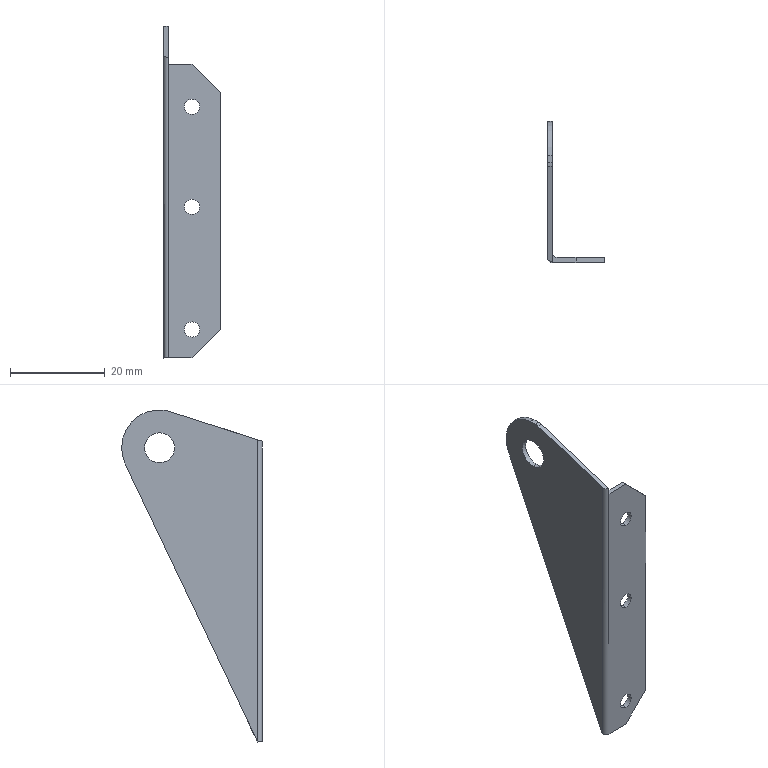Part | SolidWorks | features BaseBody 1 | 1 solid | 24 faces | box 12 x 29.68 x 70 mm | volume 1722 mm3 | cylinder 12 | plane 12 | commonest cylinder face diameters 3.2 x6 2 x2 6.35 x2 16 x2
STEP:
#1=CARTESIAN_POINT('',(6.,0.,33.461));
#2=VERTEX_POINT('',#1);
#3=CARTESIAN_POINT('',(6.,0.,30.261));
#4=VERTEX_POINT('',#3);
#5=CARTESIAN_POINT('',(6.,0.,31.861));
#6=DIRECTION('',(0.,-1.,0.));
#7=DIRECTION('',(0.,0.,1.));
#8=AXIS2_PLACEMENT_3D('',#5,#6,#7);
#9=CIRCLE('',#8,1.6);
#10=EDGE_CURVE('',#2,#4,#9,.T.);
#11=ORIENTED_EDGE('',*,*,#10,.T.);
#12=CARTESIAN_POINT('',(6.,1.,30.261));
#13=VERTEX_POINT('',#12);
#14=CARTESIAN_POINT('',(6.,0.,30.261));
#15=DIRECTION('',(0.,1.,0.));
#16=VECTOR('',#15,1000.);
#17=LINE('',#14,#16);
#18=EDGE_CURVE('',#4,#13,#17,.T.);
#19=ORIENTED_EDGE('',*,*,#18,.T.);
#20=CARTESIAN_POINT('',(6.,1.,33.461));
#21=VERTEX_POINT('',#20);
#22=CARTESIAN_POINT('',(6.,1.,31.861));
#23=DIRECTION('',(0.,1.,0.));
#24=DIRECTION('',(0.,0.,1.));
#25=AXIS2_PLACEMENT_3D('',#22,#23,#24);
#26=CIRCLE('',#25,1.6);
#27=EDGE_CURVE('',#13,#21,#26,.T.);
#28=ORIENTED_EDGE('',*,*,#27,.T.);
#29=CARTESIAN_POINT('',(6.,0.,33.461));
#30=DIRECTION('',(0.,1.,0.));
#31=VECTOR('',#30,1000.);
#32=LINE('',#29,#31);
#33=EDGE_CURVE('',#2,#21,#32,.T.);
#34=ORIENTED_EDGE('',*,*,#33,.F.);
#35=EDGE_LOOP('',(#11,#19,#28,#34));
#36=FACE_OUTER_BOUND('',#35,.T.);
#37=CARTESIAN_POINT('',(6.,0.,31.861));
#38=DIRECTION('',(0.,1.,0.));
#39=DIRECTION('',(0.,0.,1.));
#40=AXIS2_PLACEMENT_3D('',#37,#38,#39);
#41=CYLINDRICAL_SURFACE('',#40,1.6);
#42=ADVANCED_FACE('',(#36),#41,.F.);
#43=CARTESIAN_POINT('',(6.,0.,54.587));
#44=VERTEX_POINT('',#43);
#45=CARTESIAN_POINT('',(6.,0.,51.387));
#46=VERTEX_POINT('',#45);
#47=CARTESIAN_POINT('',(6.,0.,52.987));
#48=DIRECTION('',(0.,-1.,0.));
#49=DIRECTION('',(0.,0.,1.));
#50=AXIS2_PLACEMENT_3D('',#47,#48,#49);
#51=CIRCLE('',#50,1.6);
#52=EDGE_CURVE('',#44,#46,#51,.T.);
#53=ORIENTED_EDGE('',*,*,#52,.T.);
#54=CARTESIAN_POINT('',(6.,1.,51.387));
#55=VERTEX_POINT('',#54);
#56=CARTESIAN_POINT('',(6.,0.,51.387));
#57=DIRECTION('',(0.,1.,0.));
#58=VECTOR('',#57,1000.);
#59=LINE('',#56,#58);
#60=EDGE_CURVE('',#46,#55,#59,.T.);
#61=ORIENTED_EDGE('',*,*,#60,.T.);
#62=CARTESIAN_POINT('',(6.,1.,54.587));
#63=VERTEX_POINT('',#62);
#64=CARTESIAN_POINT('',(6.,1.,52.987));
#65=DIRECTION('',(0.,1.,0.));
#66=DIRECTION('',(0.,0.,1.));
#67=AXIS2_PLACEMENT_3D('',#64,#65,#66);
#68=CIRCLE('',#67,1.6);
#69=EDGE_CURVE('',#55,#63,#68,.T.);
#70=ORIENTED_EDGE('',*,*,#69,.T.);
#71=CARTESIAN_POINT('',(6.,0.,54.587));
#72=DIRECTION('',(0.,1.,0.));
#73=VECTOR('',#72,1000.);
#74=LINE('',#71,#73);
#75=EDGE_CURVE('',#44,#63,#74,.T.);
#76=ORIENTED_EDGE('',*,*,#75,.F.);
#77=EDGE_LOOP('',(#53,#61,#70,#76));
#78=FACE_OUTER_BOUND('',#77,.T.);
#79=CARTESIAN_POINT('',(6.,0.,52.987));
#80=DIRECTION('',(0.,1.,0.));
#81=DIRECTION('',(0.,0.,1.));
#82=AXIS2_PLACEMENT_3D('',#79,#80,#81);
#83=CYLINDRICAL_SURFACE('',#82,1.6);
#84=ADVANCED_FACE('',(#78),#83,.F.);
#85=CARTESIAN_POINT('',(6.,0.,7.6));
#86=VERTEX_POINT('',#85);
#87=CARTESIAN_POINT('',(6.,0.,4.4));
#88=VERTEX_POINT('',#87);
#89=CARTESIAN_POINT('',(6.,0.,6.));
#90=DIRECTION('',(0.,-1.,0.));
#91=DIRECTION('',(0.,0.,1.));
#92=AXIS2_PLACEMENT_3D('',#89,#90,#91);
#93=CIRCLE('',#92,1.6);
#94=EDGE_CURVE('',#86,#88,#93,.T.);
#95=ORIENTED_EDGE('',*,*,#94,.T.);
#96=CARTESIAN_POINT('',(6.,1.,4.4));
#97=VERTEX_POINT('',#96);
#98=CARTESIAN_POINT('',(6.,0.,4.4));
#99=DIRECTION('',(0.,1.,0.));
#100=VECTOR('',#99,1000.);
#101=LINE('',#98,#100);
#102=EDGE_CURVE('',#88,#97,#101,.T.);
#103=ORIENTED_EDGE('',*,*,#102,.T.);
#104=CARTESIAN_POINT('',(6.,1.,7.6));
#105=VERTEX_POINT('',#104);
#106=CARTESIAN_POINT('',(6.,1.,6.));
#107=DIRECTION('',(0.,1.,0.));
#108=DIRECTION('',(0.,0.,1.));
#109=AXIS2_PLACEMENT_3D('',#106,#107,#108);
#110=CIRCLE('',#109,1.6);
#111=EDGE_CURVE('',#97,#105,#110,.T.);
#112=ORIENTED_EDGE('',*,*,#111,.T.);
#113=CARTESIAN_POINT('',(6.,0.,7.6));
#114=DIRECTION('',(0.,1.,0.));
#115=VECTOR('',#114,1000.);
#116=LINE('',#113,#115);
#117=EDGE_CURVE('',#86,#105,#116,.T.);
#118=ORIENTED_EDGE('',*,*,#117,.F.);
#119=EDGE_LOOP('',(#95,#103,#112,#118));
#120=FACE_OUTER_BOUND('',#119,.T.);
#121=CARTESIAN_POINT('',(6.,0.,6.));
#122=DIRECTION('',(0.,1.,0.));
#123=DIRECTION('',(0.,0.,1.));
#124=AXIS2_PLACEMENT_3D('',#121,#122,#123);
#125=CYLINDRICAL_SURFACE('',#124,1.6);
#126=ADVANCED_FACE('',(#120),#125,.F.);
#127=CARTESIAN_POINT('',(0.,21.68,58.856));
#128=VERTEX_POINT('',#127);
#129=CARTESIAN_POINT('',(0.,21.68,65.206));
#130=VERTEX_POINT('',#129);
#131=CARTESIAN_POINT('',(0.,21.68,62.031));
#132=DIRECTION('',(-1.,0.,0.));
#133=DIRECTION('',(0.,0.,-1.));
#134=AXIS2_PLACEMENT_3D('',#131,#132,#133);
#135=CIRCLE('',#134,3.175);
#136=EDGE_CURVE('',#128,#130,#135,.T.);
#137=ORIENTED_EDGE('',*,*,#136,.T.);
#138=CARTESIAN_POINT('',(1.,21.68,65.206));
#139=VERTEX_POINT('',#138);
#140=CARTESIAN_POINT('',(0.,21.68,65.206));
#141=DIRECTION('',(1.,0.,0.));
#142=VECTOR('',#141,1000.);
#143=LINE('',#140,#142);
#144=EDGE_CURVE('',#130,#139,#143,.T.);
#145=ORIENTED_EDGE('',*,*,#144,.T.);
#146=CARTESIAN_POINT('',(1.,21.68,58.856));
#147=VERTEX_POINT('',#146);
#148=CARTESIAN_POINT('',(1.,21.68,62.031));
#149=DIRECTION('',(1.,0.,0.));
#150=DIRECTION('',(0.,0.,-1.));
#151=AXIS2_PLACEMENT_3D('',#148,#149,#150);
#152=CIRCLE('',#151,3.175);
#153=EDGE_CURVE('',#139,#147,#152,.T.);
#154=ORIENTED_EDGE('',*,*,#153,.T.);
#155=CARTESIAN_POINT('',(0.,21.68,58.856));
#156=DIRECTION('',(1.,0.,0.));
#157=VECTOR('',#156,1000.);
#158=LINE('',#155,#157);
#159=EDGE_CURVE('',#128,#147,#158,.T.);
#160=ORIENTED_EDGE('',*,*,#159,.F.);
#161=EDGE_LOOP('',(#137,#145,#154,#160));
#162=FACE_OUTER_BOUND('',#161,.T.);
#163=CARTESIAN_POINT('',(0.,21.68,62.031));
#164=DIRECTION('',(1.,0.,0.));
#165=DIRECTION('',(0.,0.,-1.));
#166=AXIS2_PLACEMENT_3D('',#163,#164,#165);
#167=CYLINDRICAL_SURFACE('',#166,3.175);
#168=ADVANCED_FACE('',(#162),#167,.F.);
#169=ORIENTED_EDGE('',*,*,#18,.F.);
#170=CARTESIAN_POINT('',(6.,0.,31.861));
#171=DIRECTION('',(0.,-1.,0.));
#172=DIRECTION('',(0.,0.,1.));
#173=AXIS2_PLACEMENT_3D('',#170,#171,#172);
#174=CIRCLE('',#173,1.6);
#175=EDGE_CURVE('',#4,#2,#174,.T.);
#176=ORIENTED_EDGE('',*,*,#175,.T.);
#177=ORIENTED_EDGE('',*,*,#33,.T.);
#178=CARTESIAN_POINT('',(6.,1.,31.861));
#179=DIRECTION('',(0.,1.,0.));
#180=DIRECTION('',(0.,0.,1.));
#181=AXIS2_PLACEMENT_3D('',#178,#179,#180);
#182=CIRCLE('',#181,1.6);
#183=EDGE_CURVE('',#21,#13,#182,.T.);
#184=ORIENTED_EDGE('',*,*,#183,.T.);
#185=EDGE_LOOP('',(#169,#176,#177,#184));
#186=FACE_OUTER_BOUND('',#185,.T.);
#187=CARTESIAN_POINT('',(6.,0.,31.861));
#188=DIRECTION('',(0.,1.,0.));
#189=DIRECTION('',(0.,0.,1.));
#190=AXIS2_PLACEMENT_3D('',#187,#188,#189);
#191=CYLINDRICAL_SURFACE('',#190,1.6);
#192=ADVANCED_FACE('',(#186),#191,.F.);
#193=CARTESIAN_POINT('',(6.,1.,52.987));
#194=DIRECTION('',(0.,1.,0.));
#195=DIRECTION('',(0.,0.,1.));
#196=AXIS2_PLACEMENT_3D('',#193,#194,#195);
#197=CIRCLE('',#196,1.6);
#198=EDGE_CURVE('',#63,#55,#197,.T.);
#199=ORIENTED_EDGE('',*,*,#198,.F.);
#200=ORIENTED_EDGE('',*,*,#69,.F.);
#201=EDGE_LOOP('',(#199,#200));
#202=FACE_BOUND('',#201,.T.);
#203=CARTESIAN_POINT('',(6.,1.,6.));
#204=DIRECTION('',(0.,1.,0.));
#205=DIRECTION('',(0.,0.,1.));
#206=AXIS2_PLACEMENT_3D('',#203,#204,#205);
#207=CIRCLE('',#206,1.6);
#208=EDGE_CURVE('',#105,#97,#207,.T.);
#209=ORIENTED_EDGE('',*,*,#208,.F.);
#210=ORIENTED_EDGE('',*,*,#111,.F.);
#211=EDGE_LOOP('',(#209,#210));
#212=FACE_BOUND('',#211,.T.);
#213=ORIENTED_EDGE('',*,*,#183,.F.);
#214=ORIENTED_EDGE('',*,*,#27,.F.);
#215=EDGE_LOOP('',(#213,#214));
#216=FACE_BOUND('',#215,.T.);
#217=CARTESIAN_POINT('',(2.,1.,61.987));
#218=VERTEX_POINT('',#217);
#219=CARTESIAN_POINT('',(2.,1.,0.));
#220=VERTEX_POINT('',#219);
#221=CARTESIAN_POINT('',(2.,1.,30.994));
#222=DIRECTION('',(0.,0.,-1.));
#223=VECTOR('',#222,1000.);
#224=LINE('',#221,#223);
#225=EDGE_CURVE('',#218,#220,#224,.T.);
#226=ORIENTED_EDGE('',*,*,#225,.F.);
#227=CARTESIAN_POINT('',(6.,1.,61.987));
#228=VERTEX_POINT('',#227);
#229=CARTESIAN_POINT('',(7.,1.,61.987));
#230=DIRECTION('',(-1.,0.,0.));
#231=VECTOR('',#230,1000.);
#232=LINE('',#229,#231);
#233=EDGE_CURVE('',#228,#218,#232,.T.);
#234=ORIENTED_EDGE('',*,*,#233,.F.);
#235=CARTESIAN_POINT('',(12.,1.,55.987));
#236=VERTEX_POINT('',#235);
#237=CARTESIAN_POINT('',(12.,1.,55.987));
#238=DIRECTION('',(-0.7071,0.,0.7071));
#239=VECTOR('',#238,1000.);
#240=LINE('',#237,#239);
#241=EDGE_CURVE('',#236,#228,#240,.T.);
#242=ORIENTED_EDGE('',*,*,#241,.F.);
#243=CARTESIAN_POINT('',(12.,1.,6.));
#244=VERTEX_POINT('',#243);
#245=CARTESIAN_POINT('',(12.,1.,30.994));
#246=DIRECTION('',(0.,0.,1.));
#247=VECTOR('',#246,1000.);
#248=LINE('',#245,#247);
#249=EDGE_CURVE('',#244,#236,#248,.T.);
#250=ORIENTED_EDGE('',*,*,#249,.F.);
#251=CARTESIAN_POINT('',(6.,1.,0.));
#252=VERTEX_POINT('',#251);
#253=CARTESIAN_POINT('',(6.,1.,0.));
#254=DIRECTION('',(0.7071,0.,0.7071));
#255=VECTOR('',#254,1000.);
#256=LINE('',#253,#255);
#257=EDGE_CURVE('',#252,#244,#256,.T.);
#258=ORIENTED_EDGE('',*,*,#257,.F.);
#259=CARTESIAN_POINT('',(7.,1.,0.));
#260=DIRECTION('',(1.,0.,0.));
#261=VECTOR('',#260,1000.);
#262=LINE('',#259,#261);
#263=EDGE_CURVE('',#220,#252,#262,.T.);
#264=ORIENTED_EDGE('',*,*,#263,.F.);
#265=EDGE_LOOP('',(#226,#234,#242,#250,#258,#264));
#266=FACE_OUTER_BOUND('',#265,.T.);
#267=CARTESIAN_POINT('',(2.,1.,61.987));
#268=DIRECTION('',(0.,-1.,0.));
#269=DIRECTION('',(0.,0.,-1.));
#270=AXIS2_PLACEMENT_3D('',#267,#268,#269);
#271=PLANE('',#270);
#272=ADVANCED_FACE('',(#202,#212,#216,#266),#271,.F.);
#273=ORIENTED_EDGE('',*,*,#52,.F.);
#274=CARTESIAN_POINT('',(6.,0.,52.987));
#275=DIRECTION('',(0.,-1.,0.));
#276=DIRECTION('',(0.,0.,1.));
#277=AXIS2_PLACEMENT_3D('',#274,#275,#276);
#278=CIRCLE('',#277,1.6);
#279=EDGE_CURVE('',#46,#44,#278,.T.);
#280=ORIENTED_EDGE('',*,*,#279,.F.);
#281=EDGE_LOOP('',(#273,#280));
#282=FACE_BOUND('',#281,.T.);
#283=ORIENTED_EDGE('',*,*,#94,.F.);
#284=CARTESIAN_POINT('',(6.,0.,6.));
#285=DIRECTION('',(0.,-1.,0.));
#286=DIRECTION('',(0.,0.,1.));
#287=AXIS2_PLACEMENT_3D('',#284,#285,#286);
#288=CIRCLE('',#287,1.6);
#289=EDGE_CURVE('',#88,#86,#288,.T.);
#290=ORIENTED_EDGE('',*,*,#289,.F.);
#291=EDGE_LOOP('',(#283,#290));
#292=FACE_BOUND('',#291,.T.);
#293=ORIENTED_EDGE('',*,*,#10,.F.);
#294=ORIENTED_EDGE('',*,*,#175,.F.);
#295=EDGE_LOOP('',(#293,#294));
#296=FACE_BOUND('',#295,.T.);
#297=CARTESIAN_POINT('',(1.,0.,0.));
#298=VERTEX_POINT('',#297);
#299=CARTESIAN_POINT('',(1.,0.,61.987));
#300=VERTEX_POINT('',#299);
#301=CARTESIAN_POINT('',(1.,0.,30.994));
#302=DIRECTION('',(0.,0.,1.));
#303=VECTOR('',#302,1000.);
#304=LINE('',#301,#303);
#305=EDGE_CURVE('',#298,#300,#304,.T.);
#306=ORIENTED_EDGE('',*,*,#305,.F.);
#307=CARTESIAN_POINT('',(6.,0.,0.));
#308=VERTEX_POINT('',#307);
#309=CARTESIAN_POINT('',(6.5,0.,0.));
#310=DIRECTION('',(-1.,0.,0.));
#311=VECTOR('',#310,1000.);
#312=LINE('',#309,#311);
#313=EDGE_CURVE('',#308,#298,#312,.T.);
#314=ORIENTED_EDGE('',*,*,#313,.F.);
#315=CARTESIAN_POINT('',(12.,0.,6.));
#316=VERTEX_POINT('',#315);
#317=CARTESIAN_POINT('',(6.,0.,0.));
#318=DIRECTION('',(-0.7071,0.,-0.7071));
#319=VECTOR('',#318,1000.);
#320=LINE('',#317,#319);
#321=EDGE_CURVE('',#316,#308,#320,.T.);
#322=ORIENTED_EDGE('',*,*,#321,.F.);
#323=CARTESIAN_POINT('',(12.,0.,55.987));
#324=VERTEX_POINT('',#323);
#325=CARTESIAN_POINT('',(12.,0.,30.994));
#326=DIRECTION('',(0.,0.,-1.));
#327=VECTOR('',#326,1000.);
#328=LINE('',#325,#327);
#329=EDGE_CURVE('',#324,#316,#328,.T.);
#330=ORIENTED_EDGE('',*,*,#329,.F.);
#331=CARTESIAN_POINT('',(6.,0.,61.987));
#332=VERTEX_POINT('',#331);
#333=CARTESIAN_POINT('',(12.,0.,55.987));
#334=DIRECTION('',(0.7071,0.,-0.7071));
#335=VECTOR('',#334,1000.);
#336=LINE('',#333,#335);
#337=EDGE_CURVE('',#332,#324,#336,.T.);
#338=ORIENTED_EDGE('',*,*,#337,.F.);
#339=CARTESIAN_POINT('',(6.5,0.,61.987));
#340=DIRECTION('',(1.,0.,0.));
#341=VECTOR('',#340,1000.);
#342=LINE('',#339,#341);
#343=EDGE_CURVE('',#300,#332,#342,.T.);
#344=ORIENTED_EDGE('',*,*,#343,.F.);
#345=EDGE_LOOP('',(#306,#314,#322,#330,#338,#344));
#346=FACE_OUTER_BOUND('',#345,.T.);
#347=CARTESIAN_POINT('',(1.,0.,0.));
#348=DIRECTION('',(0.,1.,0.));
#349=DIRECTION('',(0.,0.,1.));
#350=AXIS2_PLACEMENT_3D('',#347,#348,#349);
#351=PLANE('',#350);
#352=ADVANCED_FACE('',(#282,#292,#296,#346),#351,.F.);
#353=ORIENTED_EDGE('',*,*,#60,.F.);
#354=ORIENTED_EDGE('',*,*,#279,.T.);
#355=ORIENTED_EDGE('',*,*,#75,.T.);
#356=ORIENTED_EDGE('',*,*,#198,.T.);
#357=EDGE_LOOP('',(#353,#354,#355,#356));
#358=FACE_OUTER_BOUND('',#357,.T.);
#359=CARTESIAN_POINT('',(6.,0.,52.987));
#360=DIRECTION('',(0.,1.,0.));
#361=DIRECTION('',(0.,0.,1.));
#362=AXIS2_PLACEMENT_3D('',#359,#360,#361);
#363=CYLINDRICAL_SURFACE('',#362,1.6);
#364=ADVANCED_FACE('',(#358),#363,.F.);
#365=ORIENTED_EDGE('',*,*,#102,.F.);
#366=ORIENTED_EDGE('',*,*,#289,.T.);
#367=ORIENTED_EDGE('',*,*,#117,.T.);
#368=ORIENTED_EDGE('',*,*,#208,.T.);
#369=EDGE_LOOP('',(#365,#366,#367,#368));
#370=FACE_OUTER_BOUND('',#369,.T.);
#371=CARTESIAN_POINT('',(6.,0.,6.));
#372=DIRECTION('',(0.,1.,0.));
#373=DIRECTION('',(0.,0.,1.));
#374=AXIS2_PLACEMENT_3D('',#371,#372,#373);
#375=CYLINDRICAL_SURFACE('',#374,1.6);
#376=ADVANCED_FACE('',(#370),#375,.F.);
#377=ORIENTED_EDGE('',*,*,#263,.T.);
#378=CARTESIAN_POINT('',(6.,0.5,0.));
#379=DIRECTION('',(0.,-1.,0.));
#380=VECTOR('',#379,1000.);
#381=LINE('',#378,#380);
#382=EDGE_CURVE('',#252,#308,#381,.T.);
#383=ORIENTED_EDGE('',*,*,#382,.T.);
#384=ORIENTED_EDGE('',*,*,#313,.T.);
#385=CARTESIAN_POINT('',(0.,1.,0.));
#386=VERTEX_POINT('',#385);
#387=CARTESIAN_POINT('',(1.,1.,0.));
#388=DIRECTION('',(0.,0.,-1.));
#389=DIRECTION('',(0.,1.,0.));
#390=AXIS2_PLACEMENT_3D('',#387,#388,#389);
#391=CIRCLE('',#390,1.);
#392=EDGE_CURVE('',#298,#386,#391,.T.);
#393=ORIENTED_EDGE('',*,*,#392,.T.);
#394=CARTESIAN_POINT('',(2.982,1.,0.));
#395=DIRECTION('',(1.,0.,0.));
#396=VECTOR('',#395,1000.);
#397=LINE('',#394,#396);
#398=EDGE_CURVE('',#386,#220,#397,.T.);
#399=ORIENTED_EDGE('',*,*,#398,.T.);
#400=EDGE_LOOP('',(#377,#383,#384,#393,#399));
#401=FACE_OUTER_BOUND('',#400,.T.);
#402=CARTESIAN_POINT('',(6.,0.,0.));
#403=DIRECTION('',(0.,0.,-1.));
#404=DIRECTION('',(-1.,0.,0.));
#405=AXIS2_PLACEMENT_3D('',#402,#403,#404);
#406=PLANE('',#405);
#407=ADVANCED_FACE('',(#401),#406,.T.);
#408=CARTESIAN_POINT('',(1.,2.,2.1));
#409=VERTEX_POINT('',#408);
#410=CARTESIAN_POINT('',(2.,1.,0.));
#411=CARTESIAN_POINT('',(1.414,1.,0.000000002));
#412=CARTESIAN_POINT('',(1.,1.414,0.8699));
#413=CARTESIAN_POINT('',(1.,2.,2.1));
#414=(BOUNDED_CURVE()B_SPLINE_CURVE(3,(#410,#411,#412,#413),.UNSPECIFIED.,.F.,.F.)B_SPLINE_CURVE_WITH_KNOTS((4,4),(3.142,4.712),.UNSPECIFIED.)CURVE()GEOMETRIC_REPRESENTATION_ITEM()RATIONAL_B_SPLINE_CURVE((1.,0.8047,0.8047,1.))REPRESENTATION_ITEM(''));
#415=EDGE_CURVE('',#220,#409,#414,.T.);
#416=ORIENTED_EDGE('',*,*,#415,.T.);
#417=CARTESIAN_POINT('',(1.,2.,61.987));
#418=VERTEX_POINT('',#417);
#419=CARTESIAN_POINT('',(1.,2.,30.808));
#420=DIRECTION('',(0.,0.,1.));
#421=VECTOR('',#420,1000.);
#422=LINE('',#419,#421);
#423=EDGE_CURVE('',#409,#418,#422,.T.);
#424=ORIENTED_EDGE('',*,*,#423,.T.);
#425=CARTESIAN_POINT('',(2.,2.,61.987));
#426=DIRECTION('',(0.,0.,1.));
#427=DIRECTION('',(0.,-1.,0.));
#428=AXIS2_PLACEMENT_3D('',#425,#426,#427);
#429=CIRCLE('',#428,1.);
#430=EDGE_CURVE('',#418,#218,#429,.T.);
#431=ORIENTED_EDGE('',*,*,#430,.T.);
#432=ORIENTED_EDGE('',*,*,#225,.T.);
#433=EDGE_LOOP('',(#416,#424,#431,#432));
#434=FACE_OUTER_BOUND('',#433,.T.);
#435=CARTESIAN_POINT('',(2.,2.,-0.3719));
#436=DIRECTION('',(0.,0.,1.));
#437=DIRECTION('',(0.,-1.,0.));
#438=AXIS2_PLACEMENT_3D('',#435,#436,#437);
#439=CYLINDRICAL_SURFACE('',#438,1.);
#440=ADVANCED_FACE('',(#434),#439,.F.);
#441=ORIENTED_EDGE('',*,*,#233,.T.);
#442=ORIENTED_EDGE('',*,*,#430,.F.);
#443=CARTESIAN_POINT('',(1.,1.006,61.987));
#444=DIRECTION('',(0.,1.,0.));
#445=VECTOR('',#444,1000.);
#446=LINE('',#443,#445);
#447=EDGE_CURVE('',#300,#418,#446,.T.);
#448=ORIENTED_EDGE('',*,*,#447,.F.);
#449=ORIENTED_EDGE('',*,*,#343,.T.);
#450=CARTESIAN_POINT('',(6.,1.006,61.987));
#451=DIRECTION('',(0.,-1.,0.));
#452=VECTOR('',#451,1000.);
#453=LINE('',#450,#452);
#454=EDGE_CURVE('',#228,#332,#453,.T.);
#455=ORIENTED_EDGE('',*,*,#454,.F.);
#456=EDGE_LOOP('',(#441,#442,#448,#449,#455));
#457=FACE_OUTER_BOUND('',#456,.T.);
#458=CARTESIAN_POINT('',(6.,0.,61.987));
#459=DIRECTION('',(0.,0.,-1.));
#460=DIRECTION('',(-1.,0.,0.));
#461=AXIS2_PLACEMENT_3D('',#458,#459,#460);
#462=PLANE('',#461);
#463=ADVANCED_FACE('',(#457),#462,.F.);
#464=ORIENTED_EDGE('',*,*,#241,.T.);
#465=ORIENTED_EDGE('',*,*,#454,.T.);
#466=ORIENTED_EDGE('',*,*,#337,.T.);
#467=CARTESIAN_POINT('',(12.,0.5,55.987));
#468=DIRECTION('',(0.,-1.,0.));
#469=VECTOR('',#468,1000.);
#470=LINE('',#467,#469);
#471=EDGE_CURVE('',#236,#324,#470,.T.);
#472=ORIENTED_EDGE('',*,*,#471,.F.);
#473=EDGE_LOOP('',(#464,#465,#466,#472));
#474=FACE_OUTER_BOUND('',#473,.T.);
#475=CARTESIAN_POINT('',(12.,0.,55.987));
#476=DIRECTION('',(-0.7071,0.,-0.7071));
#477=DIRECTION('',(-0.7071,0.,0.7071));
#478=AXIS2_PLACEMENT_3D('',#475,#476,#477);
#479=PLANE('',#478);
#480=ADVANCED_FACE('',(#474),#479,.F.);
#481=CARTESIAN_POINT('',(12.,0.5,6.));
#482=DIRECTION('',(0.,-1.,0.));
#483=VECTOR('',#482,1000.);
#484=LINE('',#481,#483);
#485=EDGE_CURVE('',#244,#316,#484,.T.);
#486=ORIENTED_EDGE('',*,*,#485,.F.);
#487=ORIENTED_EDGE('',*,*,#249,.T.);
#488=ORIENTED_EDGE('',*,*,#471,.T.);
#489=ORIENTED_EDGE('',*,*,#329,.T.);
#490=EDGE_LOOP('',(#486,#487,#488,#489));
#491=FACE_OUTER_BOUND('',#490,.T.);
#492=CARTESIAN_POINT('',(12.,0.,6.));
#493=DIRECTION('',(-1.,0.,0.));
#494=DIRECTION('',(0.,0.,1.));
#495=AXIS2_PLACEMENT_3D('',#492,#493,#494);
#496=PLANE('',#495);
#497=ADVANCED_FACE('',(#491),#496,.F.);
#498=ORIENTED_EDGE('',*,*,#257,.T.);
#499=ORIENTED_EDGE('',*,*,#485,.T.);
#500=ORIENTED_EDGE('',*,*,#321,.T.);
#501=ORIENTED_EDGE('',*,*,#382,.F.);
#502=EDGE_LOOP('',(#498,#499,#500,#501));
#503=FACE_OUTER_BOUND('',#502,.T.);
#504=CARTESIAN_POINT('',(6.,0.,0.));
#505=DIRECTION('',(-0.7071,0.,0.7071));
#506=DIRECTION('',(0.7071,0.,0.7071));
#507=AXIS2_PLACEMENT_3D('',#504,#505,#506);
#508=PLANE('',#507);
#509=ADVANCED_FACE('',(#503),#508,.F.);
#510=CARTESIAN_POINT('',(0.,1.,63.721));
#511=VERTEX_POINT('',#510);
#512=CARTESIAN_POINT('',(0.,1.,32.052));
#513=DIRECTION('',(0.,0.,1.));
#514=VECTOR('',#513,1000.);
#515=LINE('',#512,#514);
#516=EDGE_CURVE('',#386,#511,#515,.T.);
#517=ORIENTED_EDGE('',*,*,#516,.F.);
#518=ORIENTED_EDGE('',*,*,#392,.F.);
#519=ORIENTED_EDGE('',*,*,#305,.T.);
#520=CARTESIAN_POINT('',(1.,0.,63.4));
#521=VERTEX_POINT('',#520);
#522=CARTESIAN_POINT('',(1.,0.,32.052));
#523=DIRECTION('',(0.,0.,-1.));
#524=VECTOR('',#523,1000.);
#525=LINE('',#522,#524);
#526=EDGE_CURVE('',#521,#300,#525,.T.);
#527=ORIENTED_EDGE('',*,*,#526,.F.);
#528=CARTESIAN_POINT('',(1.,0.,63.4));
#529=CARTESIAN_POINT('',(0.4142,0.,63.4));
#530=CARTESIAN_POINT('',(0.,0.4142,63.533));
#531=CARTESIAN_POINT('',(0.,1.,63.721));
#532=(BOUNDED_CURVE()B_SPLINE_CURVE(3,(#528,#529,#530,#531),.UNSPECIFIED.,.F.,.F.)B_SPLINE_CURVE_WITH_KNOTS((4,4),(6.283,7.854),.UNSPECIFIED.)CURVE()GEOMETRIC_REPRESENTATION_ITEM()RATIONAL_B_SPLINE_CURVE((1.,0.8047,0.8047,1.))REPRESENTATION_ITEM(''));
#533=EDGE_CURVE('',#521,#511,#532,.T.);
#534=ORIENTED_EDGE('',*,*,#533,.T.);
#535=EDGE_LOOP('',(#517,#518,#519,#527,#534));
#536=FACE_OUTER_BOUND('',#535,.T.);
#537=CARTESIAN_POINT('',(1.,1.,64.104));
#538=DIRECTION('',(0.,0.,-1.));
#539=DIRECTION('',(0.,1.,0.));
#540=AXIS2_PLACEMENT_3D('',#537,#538,#539);
#541=CYLINDRICAL_SURFACE('',#540,1.);
#542=ADVANCED_FACE('',(#536),#541,.T.);
#543=CARTESIAN_POINT('',(1.,28.8,58.383));
#544=VERTEX_POINT('',#543);
#545=CARTESIAN_POINT('',(1.,14.9,29.191));
#546=DIRECTION('',(0.,0.4299,0.9029));
#547=VECTOR('',#546,1000.);
#548=LINE('',#545,#547);
#549=EDGE_CURVE('',#409,#544,#548,.T.);
#550=ORIENTED_EDGE('',*,*,#549,.F.);
#551=ORIENTED_EDGE('',*,*,#415,.F.);
#552=ORIENTED_EDGE('',*,*,#398,.F.);
#553=CARTESIAN_POINT('',(0.,28.8,58.383));
#554=VERTEX_POINT('',#553);
#555=CARTESIAN_POINT('',(0.,14.9,29.191));
#556=DIRECTION('',(0.,-0.4299,-0.9029));
#557=VECTOR('',#556,1000.);
#558=LINE('',#555,#557);
#559=EDGE_CURVE('',#554,#386,#558,.T.);
#560=ORIENTED_EDGE('',*,*,#559,.F.);
#561=CARTESIAN_POINT('',(0.5,28.8,58.383));
#562=DIRECTION('',(1.,0.,0.));
#563=VECTOR('',#562,1000.);
#564=LINE('',#561,#563);
#565=EDGE_CURVE('',#554,#544,#564,.T.);
#566=ORIENTED_EDGE('',*,*,#565,.T.);
#567=EDGE_LOOP('',(#550,#551,#552,#560,#566));
#568=FACE_OUTER_BOUND('',#567,.T.);
#569=CARTESIAN_POINT('',(0.,28.8,58.383));
#570=DIRECTION('',(0.,-0.9029,0.4299));
#571=DIRECTION('',(0.,-0.4299,-0.9029));
#572=AXIS2_PLACEMENT_3D('',#569,#570,#571);
#573=PLANE('',#572);
#574=ADVANCED_FACE('',(#568),#573,.F.);
#575=CARTESIAN_POINT('',(1.,21.68,62.031));
#576=DIRECTION('',(1.,0.,0.));
#577=DIRECTION('',(0.,0.,-1.));
#578=AXIS2_PLACEMENT_3D('',#575,#576,#577);
#579=CIRCLE('',#578,3.175);
#580=EDGE_CURVE('',#147,#139,#579,.T.);
#581=ORIENTED_EDGE('',*,*,#580,.F.);
#582=ORIENTED_EDGE('',*,*,#153,.F.);
#583=EDGE_LOOP('',(#581,#582));
#584=FACE_BOUND('',#583,.T.);
#585=ORIENTED_EDGE('',*,*,#423,.F.);
#586=ORIENTED_EDGE('',*,*,#549,.T.);
#587=CARTESIAN_POINT('',(1.,22.388,70.));
#588=VERTEX_POINT('',#587);
#589=CARTESIAN_POINT('',(1.,21.68,62.031));
#590=DIRECTION('',(-1.,0.,0.));
#591=DIRECTION('',(0.,0.,-1.));
#592=AXIS2_PLACEMENT_3D('',#589,#590,#591);
#593=CIRCLE('',#592,8.);
#594=EDGE_CURVE('',#588,#544,#593,.T.);
#595=ORIENTED_EDGE('',*,*,#594,.F.);
#596=CARTESIAN_POINT('',(1.,20.972,70.));
#597=VERTEX_POINT('',#596);
#598=CARTESIAN_POINT('',(1.,14.929,70.));
#599=DIRECTION('',(0.,1.,0.));
#600=VECTOR('',#599,1000.);
#601=LINE('',#598,#600);
#602=EDGE_CURVE('',#597,#588,#601,.T.);
#603=ORIENTED_EDGE('',*,*,#602,.F.);
#604=CARTESIAN_POINT('',(1.,20.192,69.892));
#605=VERTEX_POINT('',#604);
#606=CARTESIAN_POINT('',(1.,21.68,62.031));
#607=DIRECTION('',(-1.,0.,0.));
#608=DIRECTION('',(0.,0.,-1.));
#609=AXIS2_PLACEMENT_3D('',#606,#607,#608);
#610=CIRCLE('',#609,8.);
#611=EDGE_CURVE('',#605,#597,#610,.T.);
#612=ORIENTED_EDGE('',*,*,#611,.F.);
#613=CARTESIAN_POINT('',(1.,-0.1212,63.361));
#614=DIRECTION('',(0.,0.952,0.3061));
#615=VECTOR('',#614,1000.);
#616=LINE('',#613,#615);
#617=EDGE_CURVE('',#521,#605,#616,.T.);
#618=ORIENTED_EDGE('',*,*,#617,.F.);
#619=ORIENTED_EDGE('',*,*,#526,.T.);
#620=ORIENTED_EDGE('',*,*,#447,.T.);
#621=EDGE_LOOP('',(#585,#586,#595,#603,#612,#618,#619,#620));
#622=FACE_OUTER_BOUND('',#621,.T.);
#623=CARTESIAN_POINT('',(1.,0.,1.693));
#624=DIRECTION('',(-1.,0.,0.));
#625=DIRECTION('',(0.,0.,1.));
#626=AXIS2_PLACEMENT_3D('',#623,#624,#625);
#627=PLANE('',#626);
#628=ADVANCED_FACE('',(#584,#622),#627,.F.);
#629=ORIENTED_EDGE('',*,*,#136,.F.);
#630=CARTESIAN_POINT('',(0.,21.68,62.031));
#631=DIRECTION('',(-1.,0.,0.));
#632=DIRECTION('',(0.,0.,-1.));
#633=AXIS2_PLACEMENT_3D('',#630,#631,#632);
#634=CIRCLE('',#633,3.175);
#635=EDGE_CURVE('',#130,#128,#634,.T.);
#636=ORIENTED_EDGE('',*,*,#635,.F.);
#637=EDGE_LOOP('',(#629,#636));
#638=FACE_BOUND('',#637,.T.);
#639=ORIENTED_EDGE('',*,*,#516,.T.);
#640=CARTESIAN_POINT('',(0.,20.192,69.892));
#641=VERTEX_POINT('',#640);
#642=CARTESIAN_POINT('',(0.,-0.1212,63.361));
#643=DIRECTION('',(0.,-0.952,-0.3061));
#644=VECTOR('',#643,1000.);
#645=LINE('',#642,#644);
#646=EDGE_CURVE('',#641,#511,#645,.T.);
#647=ORIENTED_EDGE('',*,*,#646,.F.);
#648=CARTESIAN_POINT('',(0.,20.972,70.));
#649=VERTEX_POINT('',#648);
#650=CARTESIAN_POINT('',(0.,21.68,62.031));
#651=DIRECTION('',(1.,0.,0.));
#652=DIRECTION('',(0.,0.,-1.));
#653=AXIS2_PLACEMENT_3D('',#650,#651,#652);
#654=CIRCLE('',#653,8.);
#655=EDGE_CURVE('',#649,#641,#654,.T.);
#656=ORIENTED_EDGE('',*,*,#655,.F.);
#657=CARTESIAN_POINT('',(0.,22.388,70.));
#658=VERTEX_POINT('',#657);
#659=CARTESIAN_POINT('',(0.,15.426,70.));
#660=DIRECTION('',(0.,-1.,0.));
#661=VECTOR('',#660,1000.);
#662=LINE('',#659,#661);
#663=EDGE_CURVE('',#658,#649,#662,.T.);
#664=ORIENTED_EDGE('',*,*,#663,.F.);
#665=CARTESIAN_POINT('',(0.,21.68,62.031));
#666=DIRECTION('',(1.,0.,0.));
#667=DIRECTION('',(0.,0.,-1.));
#668=AXIS2_PLACEMENT_3D('',#665,#666,#667);
#669=CIRCLE('',#668,8.);
#670=EDGE_CURVE('',#554,#658,#669,.T.);
#671=ORIENTED_EDGE('',*,*,#670,.F.);
#672=ORIENTED_EDGE('',*,*,#559,.T.);
#673=EDGE_LOOP('',(#639,#647,#656,#664,#671,#672));
#674=FACE_OUTER_BOUND('',#673,.T.);
#675=CARTESIAN_POINT('',(0.,1.,70.));
#676=DIRECTION('',(1.,0.,0.));
#677=DIRECTION('',(0.,0.,-1.));
#678=AXIS2_PLACEMENT_3D('',#675,#676,#677);
#679=PLANE('',#678);
#680=ADVANCED_FACE('',(#638,#674),#679,.F.);
#681=ORIENTED_EDGE('',*,*,#144,.F.);
#682=ORIENTED_EDGE('',*,*,#635,.T.);
#683=ORIENTED_EDGE('',*,*,#159,.T.);
#684=ORIENTED_EDGE('',*,*,#580,.T.);
#685=EDGE_LOOP('',(#681,#682,#683,#684));
#686=FACE_OUTER_BOUND('',#685,.T.);
#687=CARTESIAN_POINT('',(0.,21.68,62.031));
#688=DIRECTION('',(1.,0.,0.));
#689=DIRECTION('',(0.,0.,-1.));
#690=AXIS2_PLACEMENT_3D('',#687,#688,#689);
#691=CYLINDRICAL_SURFACE('',#690,3.175);
#692=ADVANCED_FACE('',(#686),#691,.F.);
#693=CARTESIAN_POINT('',(0.5,22.388,70.));
#694=DIRECTION('',(-1.,0.,0.));
#695=VECTOR('',#694,1000.);
#696=LINE('',#693,#695);
#697=EDGE_CURVE('',#588,#658,#696,.T.);
#698=ORIENTED_EDGE('',*,*,#697,.F.);
#699=ORIENTED_EDGE('',*,*,#594,.T.);
#700=ORIENTED_EDGE('',*,*,#565,.F.);
#701=ORIENTED_EDGE('',*,*,#670,.T.);
#702=EDGE_LOOP('',(#698,#699,#700,#701));
#703=FACE_OUTER_BOUND('',#702,.T.);
#704=CARTESIAN_POINT('',(0.,21.68,62.031));
#705=DIRECTION('',(1.,0.,0.));
#706=DIRECTION('',(0.,0.,-1.));
#707=AXIS2_PLACEMENT_3D('',#704,#705,#706);
#708=CYLINDRICAL_SURFACE('',#707,8.);
#709=ADVANCED_FACE('',(#703),#708,.T.);
#710=ORIENTED_EDGE('',*,*,#697,.T.);
#711=ORIENTED_EDGE('',*,*,#663,.T.);
#712=CARTESIAN_POINT('',(0.5,20.972,70.));
#713=DIRECTION('',(-1.,0.,0.));
#714=VECTOR('',#713,1000.);
#715=LINE('',#712,#714);
#716=EDGE_CURVE('',#597,#649,#715,.T.);
#717=ORIENTED_EDGE('',*,*,#716,.F.);
#718=ORIENTED_EDGE('',*,*,#602,.T.);
#719=EDGE_LOOP('',(#710,#711,#717,#718));
#720=FACE_OUTER_BOUND('',#719,.T.);
#721=CARTESIAN_POINT('',(1.,20.972,70.));
#722=DIRECTION('',(0.,0.,-1.));
#723=DIRECTION('',(-1.,0.,0.));
#724=AXIS2_PLACEMENT_3D('',#721,#722,#723);
#725=PLANE('',#724);
#726=ADVANCED_FACE('',(#720),#725,.F.);
#727=ORIENTED_EDGE('',*,*,#611,.T.);
#728=ORIENTED_EDGE('',*,*,#716,.T.);
#729=ORIENTED_EDGE('',*,*,#655,.T.);
#730=CARTESIAN_POINT('',(0.5,20.192,69.892));
#731=DIRECTION('',(-1.,0.,0.));
#732=VECTOR('',#731,1000.);
#733=LINE('',#730,#732);
#734=EDGE_CURVE('',#605,#641,#733,.T.);
#735=ORIENTED_EDGE('',*,*,#734,.F.);
#736=EDGE_LOOP('',(#727,#728,#729,#735));
#737=FACE_OUTER_BOUND('',#736,.T.);
#738=CARTESIAN_POINT('',(0.,21.68,62.031));
#739=DIRECTION('',(1.,0.,0.));
#740=DIRECTION('',(0.,0.,-1.));
#741=AXIS2_PLACEMENT_3D('',#738,#739,#740);
#742=CYLINDRICAL_SURFACE('',#741,8.);
#743=ADVANCED_FACE('',(#737),#742,.T.);
#744=ORIENTED_EDGE('',*,*,#533,.F.);
#745=ORIENTED_EDGE('',*,*,#617,.T.);
#746=ORIENTED_EDGE('',*,*,#734,.T.);
#747=ORIENTED_EDGE('',*,*,#646,.T.);
#748=EDGE_LOOP('',(#744,#745,#746,#747));
#749=FACE_OUTER_BOUND('',#748,.T.);
#750=CARTESIAN_POINT('',(0.,-0.1212,63.361));
#751=DIRECTION('',(0.,0.3061,-0.952));
#752=DIRECTION('',(0.,0.952,0.3061));
#753=AXIS2_PLACEMENT_3D('',#750,#751,#752);
#754=PLANE('',#753);
#755=ADVANCED_FACE('',(#749),#754,.F.);
#756=CLOSED_SHELL('',(#42,#84,#126,#168,#192,#272,#352,#364,#376,#407,#440,#463,#480,#497,#509,#542,#574,#628,#680,#692,#709,#726,#743,#755));
#757=MANIFOLD_SOLID_BREP('',#756);
#758=CARTESIAN_POINT('',(0.,0.,0.));
#759=DIRECTION('',(0.,0.,1.));
#760=DIRECTION('',(1.,0.,0.));
#761=AXIS2_PLACEMENT_3D('',#758,#759,#760);
#762=(LENGTH_UNIT()NAMED_UNIT(*)SI_UNIT(.MILLI.,.METRE.));
#763=UNCERTAINTY_MEASURE_WITH_UNIT(LENGTH_MEASURE(0.00001),#762,'','');
#764=(NAMED_UNIT(*)PLANE_ANGLE_UNIT()SI_UNIT($,.RADIAN.));
#765=(NAMED_UNIT(*)SI_UNIT($,.STERADIAN.)SOLID_ANGLE_UNIT());
#766=(GEOMETRIC_REPRESENTATION_CONTEXT(3)GLOBAL_UNCERTAINTY_ASSIGNED_CONTEXT((#763))GLOBAL_UNIT_ASSIGNED_CONTEXT((#762,#764,#765))REPRESENTATION_CONTEXT('',''));
#767=ADVANCED_BREP_SHAPE_REPRESENTATION('',(#757,#761),#766);